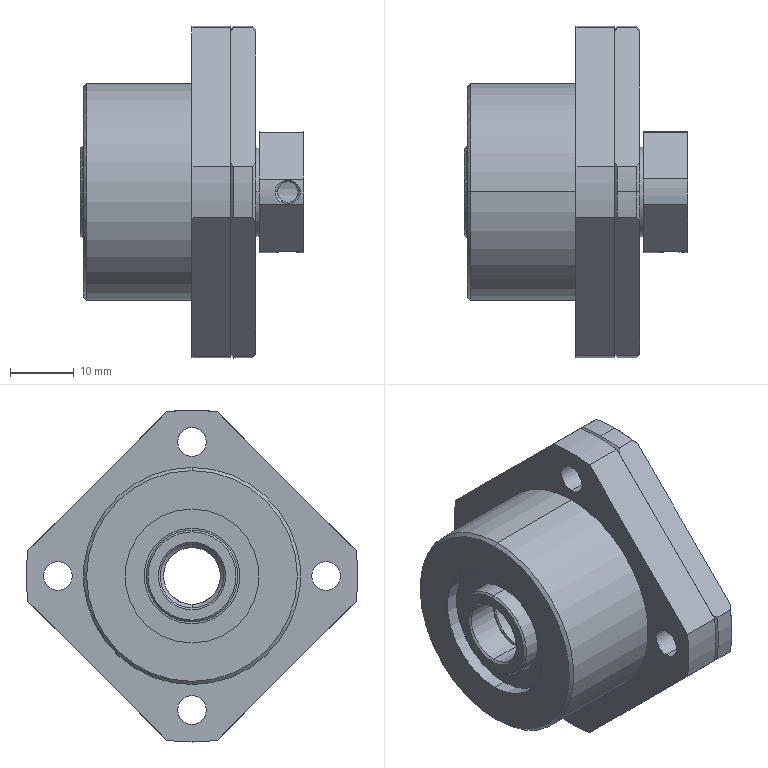Part | SolidWorks | 8 solids | 195 faces | box 35 x 52 x 52 mm | volume 28520 mm3 | cylinder 89 | cone 52 | plane 34 | spline 20 | commonest cylinder face diameters 52 x10 4.4 x8 4.5 x8 8 x8 10 x8 21 x8